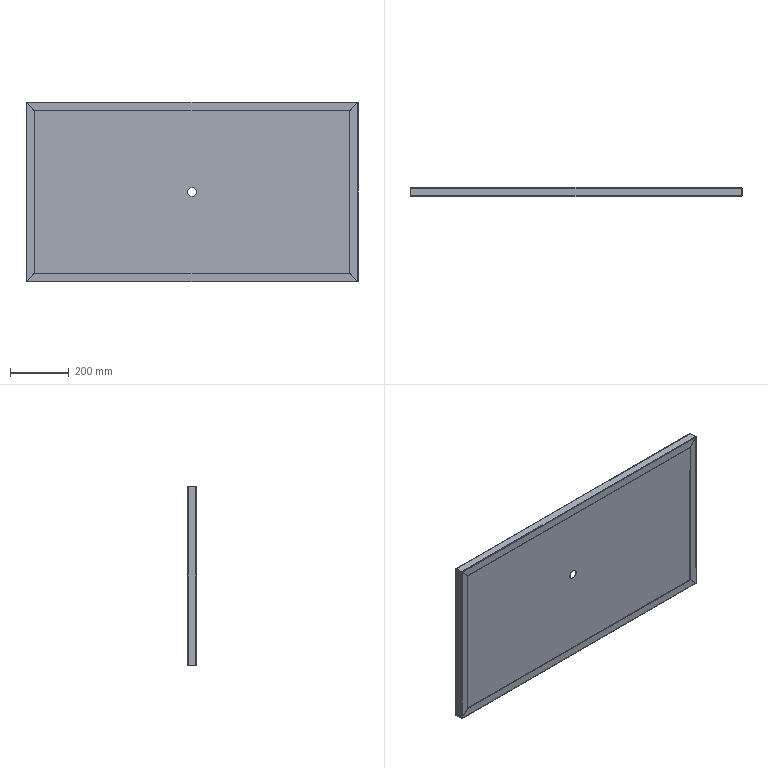Part | SolidWorks | features EdgeFlange 2, FlatPattern 1, ICE 1, SMBaseFlange 1, SheetMetal 1 | 1 solid | 72 faces | box 1135 x 30 x 615 mm | volume 1067895 mm3 | plane 38 | cylinder 18 | spline 16 | commonest cylinder face diameters 2 x8 4.4 x8 30 x2